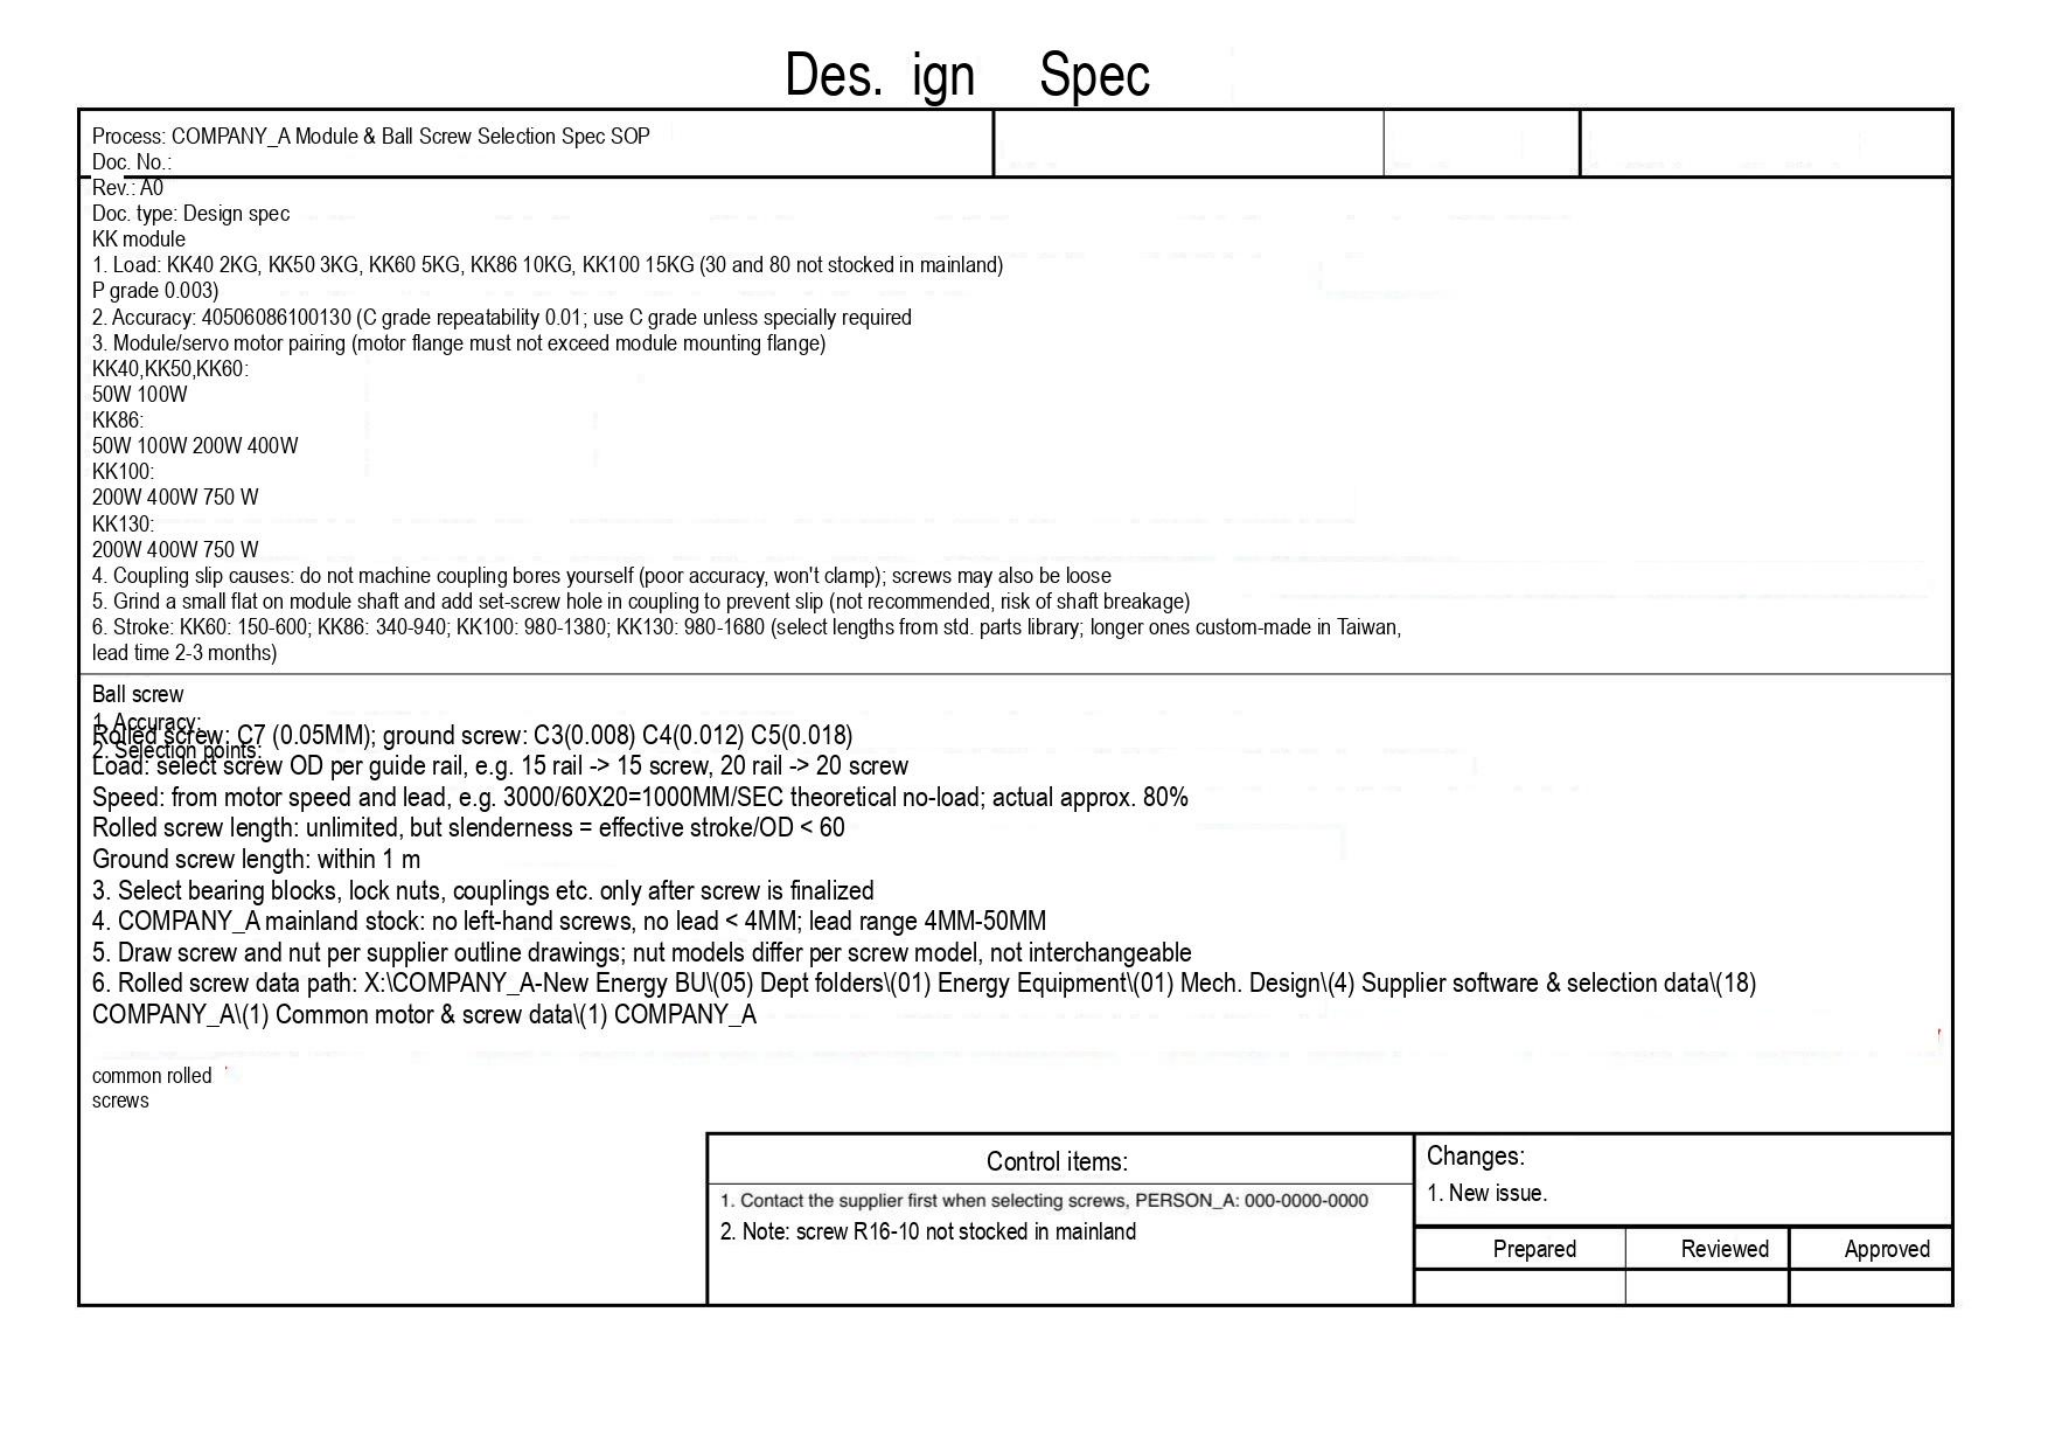# Des. ign Spec

Process: COMPANY_A Module & Ball Screw Selection Spec SOP
Doc. No.:
Rev.: A0
Doc. type: Design spec
KK module
1. Load: KK40 2KG, KK50 3KG, KK60 5KG, KK86 10KG, KK100 15KG (30 and 80 not stocked in mainland)
P grade 0.003)
2. Accuracy: 40506086100130 (C grade repeatability 0.01; use C grade unless specially required
3. Module/servo motor pairing (motor flange must not exceed module mounting flange)
KK40,KK50,KK60:
50W 100W
KK86:
50W 100W 200W 400W
KK100:
200W 400W 750 W
KK130:
200W 400W 750 W
4. Coupling slip causes: do not machine coupling bores yourself (poor accuracy, won't clamp); screws may also be loose
5. Grind a small flat on module shaft and add set-screw hole in coupling to prevent slip (not recommended, risk of shaft breakage)
6. Stroke: KK60: 150-600; KK86: 340-940; KK100: 980-1380; KK130: 980-1680 (select lengths from std. parts library; longer ones custom-made in Taiwan, lead time 2-3 months)

Ball screw
1. Accuracy:
Rolled screw: C7 (0.05MM); ground screw: C3(0.008) C4(0.012) C5(0.018)
2. Selection points:
Load: select screw OD per guide rail, e.g. 15 rail -> 15 screw, 20 rail -> 20 screw
Speed: from motor speed and lead, e.g. 3000/60X20=1000MM/SEC theoretical no-load; actual approx. 80%
Rolled screw length: unlimited, but slenderness = effective stroke/OD < 60
Ground screw length: within 1 m
3. Select bearing blocks, lock nuts, couplings etc. only after screw is finalized
4. COMPANY_A mainland stock: no left-hand screws, no lead < 4MM; lead range 4MM-50MM
5. Draw screw and nut per supplier outline drawings; nut models differ per screw model, not interchangeable
6. Rolled screw data path: X:\COMPANY_A-New Energy BU\(05) Dept folders\(01) Energy Equipment\(01) Mech. Design\(4) Supplier software & selection data\(18) COMPANY_A\(1) Common motor & screw data\(1) COMPANY_A

common rolled
screws

| Control items: |
|---|
| 1. Contact the supplier first when selecting screws, PERSON_A: 000-0000-0000 |
| 2. Note: screw R16-10 not stocked in mainland |

Changes:
1. New issue.

| Prepared | Reviewed | Approved |
|---|---|---|
| | | |